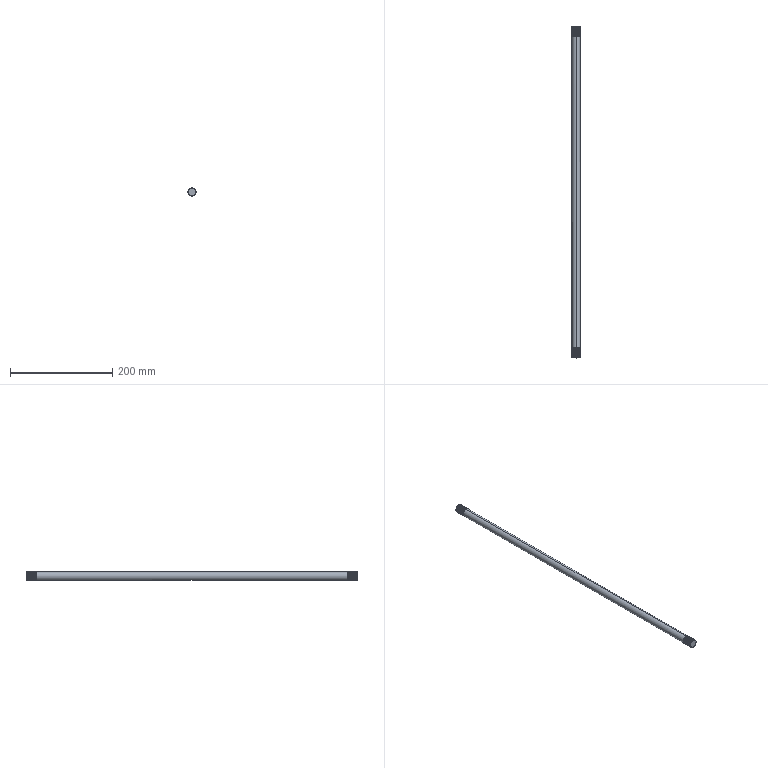Part | SolidWorks | features SweepThread 2, Extrusion 1 | 1 solid | 128 faces | box 16 x 650 x 16 mm | volume 130458 mm3 | cylinder 116 | plane 6 | spline 6 | commonest cylinder face diameters 16 x116